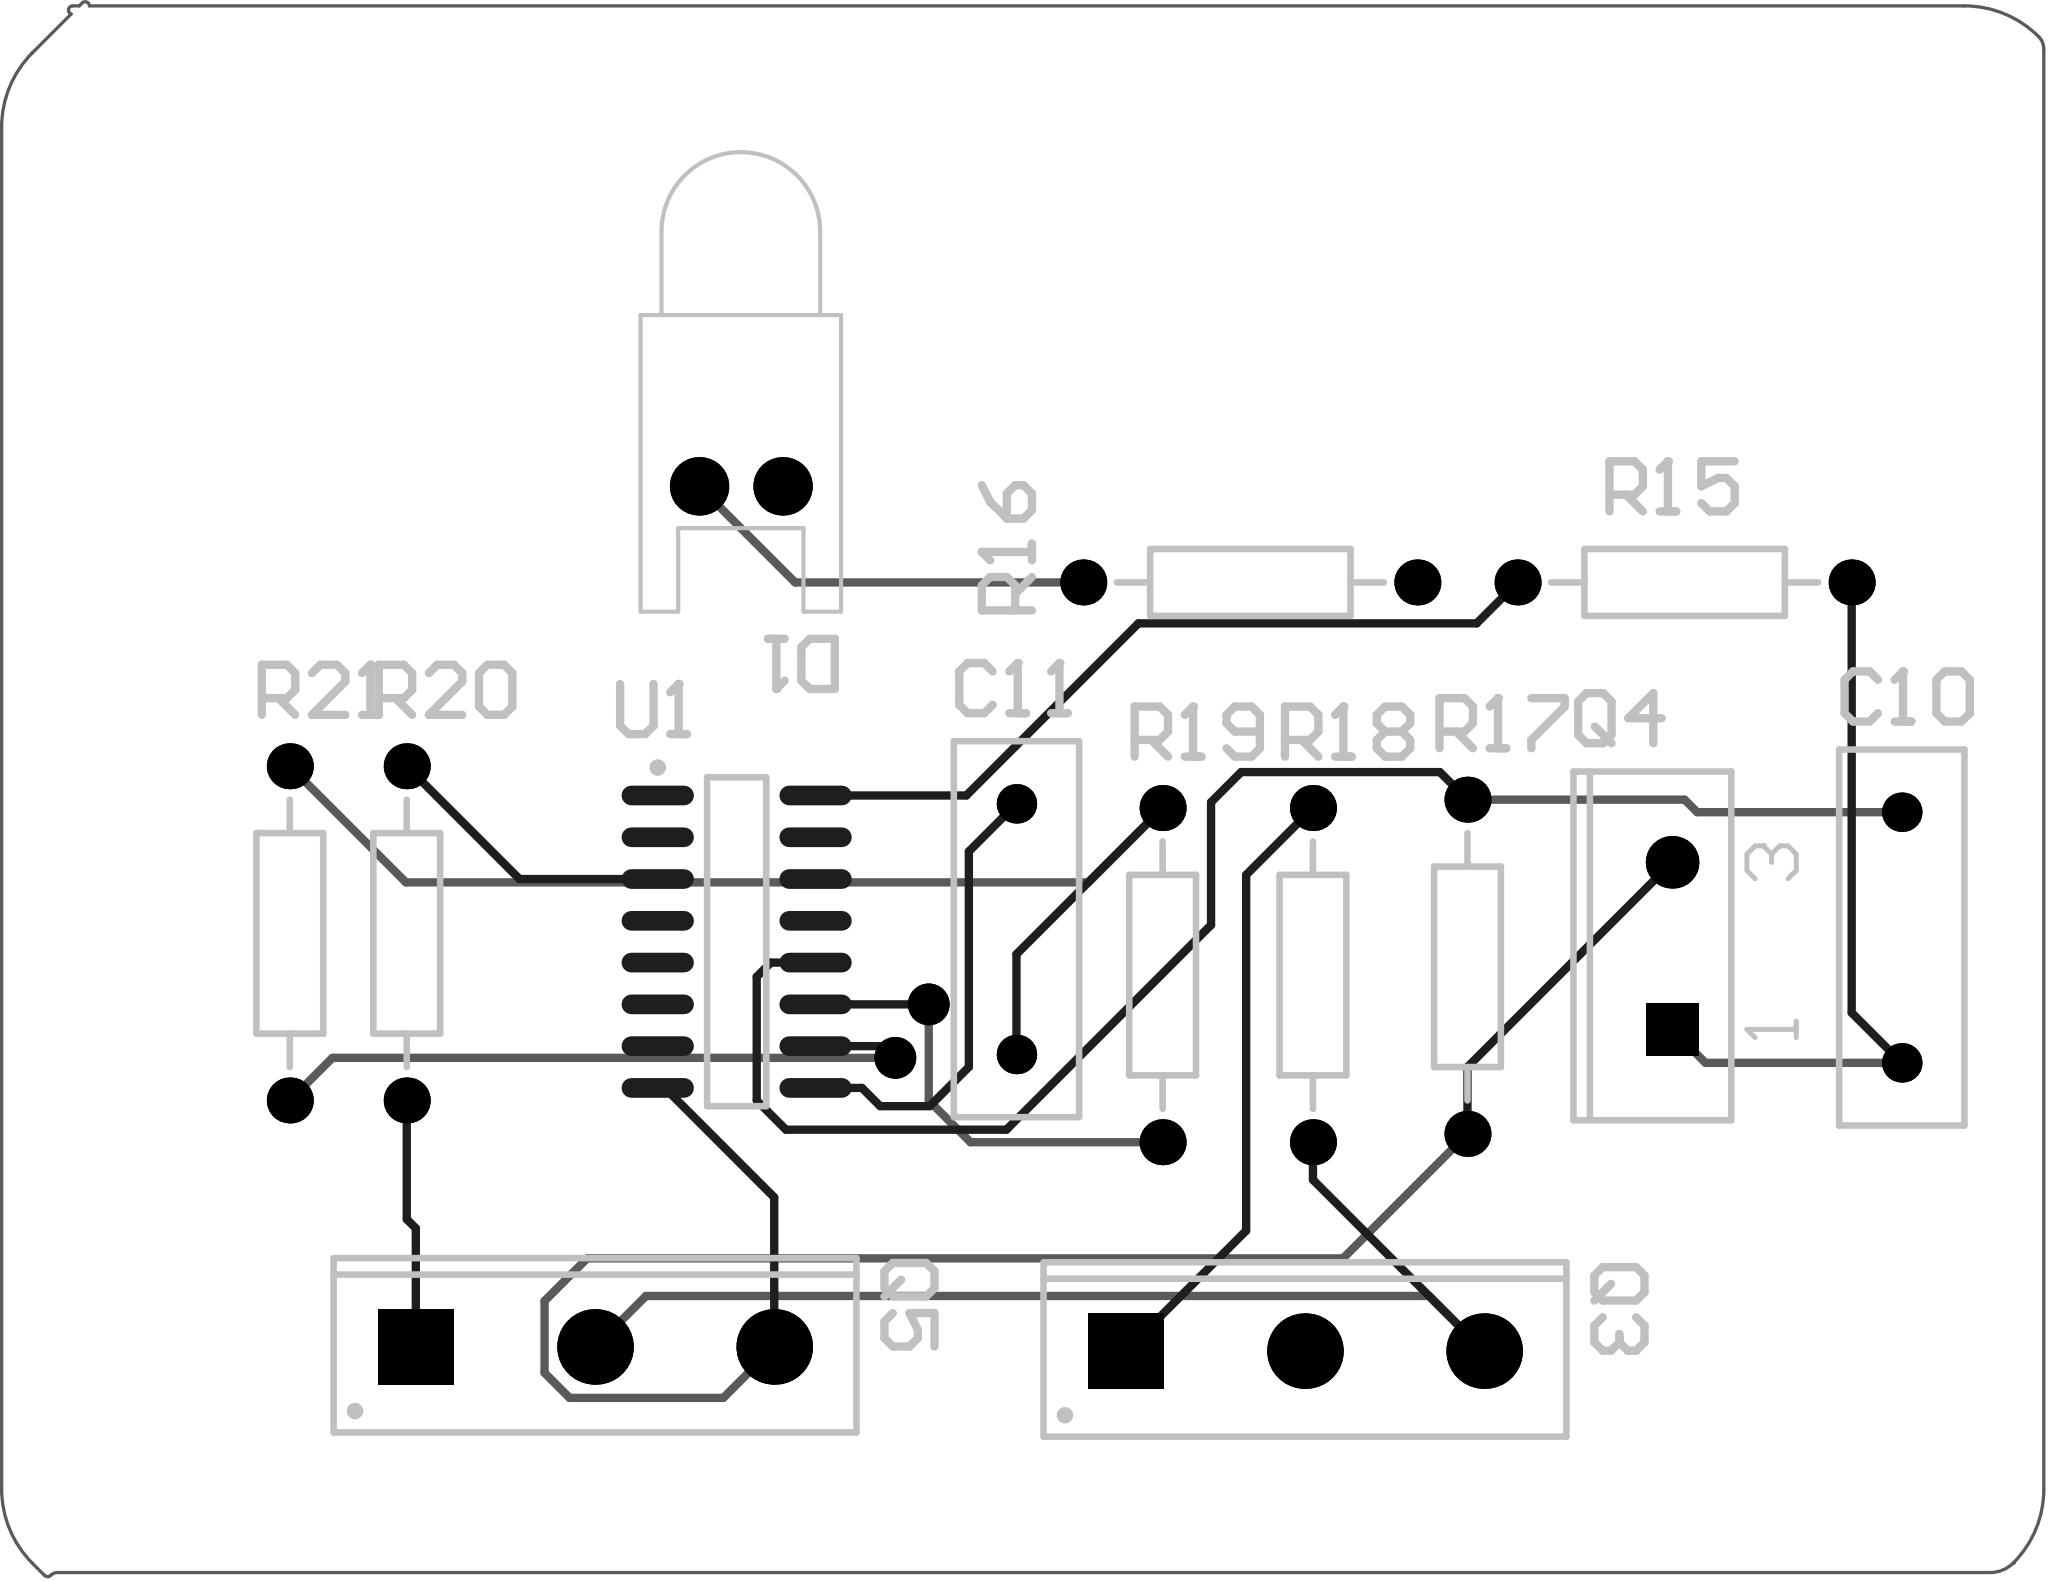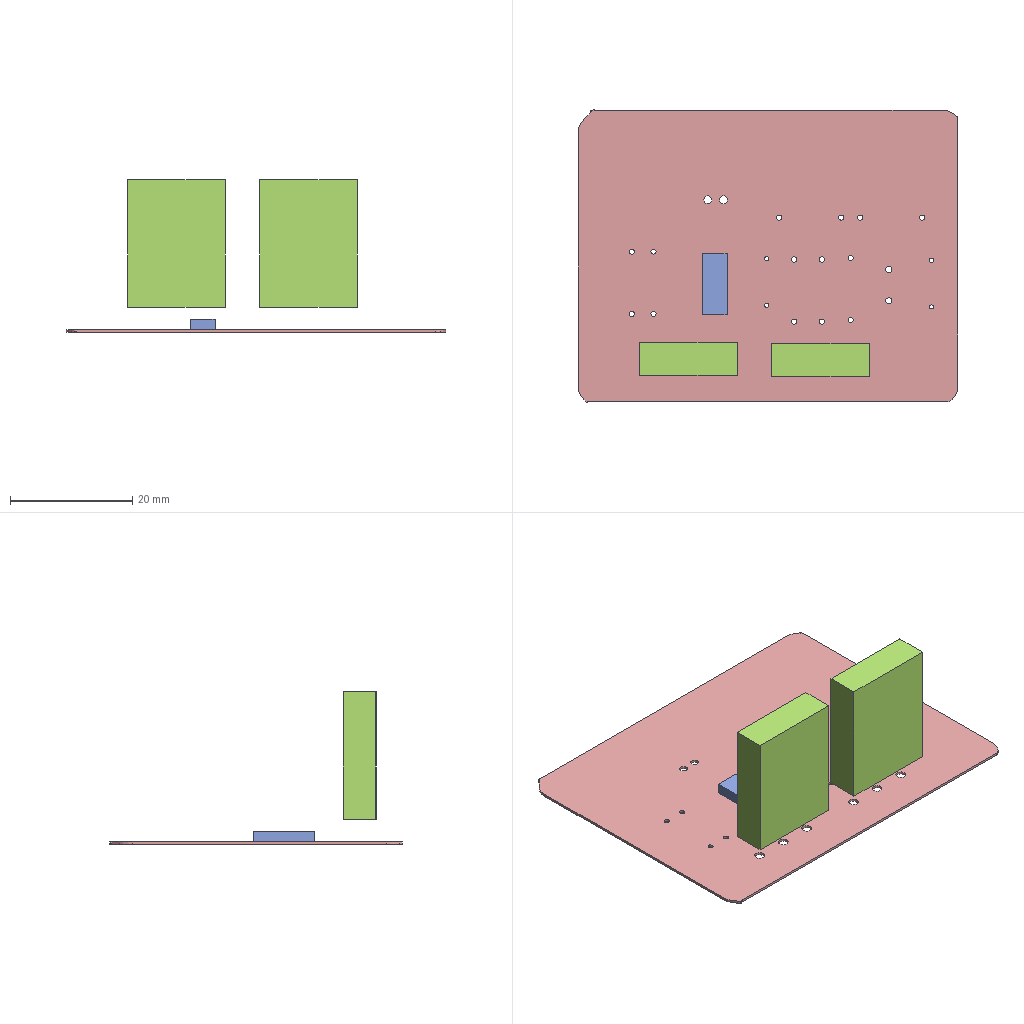Circuit board layout | Altium Designer | box 62.1 x 47.9 x 25 mm
Part placement:
Designator,Comment,Layer,Footprint,Center-X(mm),Center-Y(mm),Rotation
U1,CD4060BCM,TopLayer,M16A_N,95.504,69.85,0
R21,Res2,TopLayer,AXIAL-0.4,81.915,70.104,90
R20,Res2,TopLayer,AXIAL-0.4,85.471,70.104,90
R19,Res2,TopLayer,AXIAL-0.4,108.458,68.834,90
R18,Res2,TopLayer,AXIAL-0.4,113.03,68.834,90
R17,Res2,TopLayer,AXIAL-0.4,117.729,69.088,90
R16,Res2,TopLayer,AXIAL-0.4,111.125,80.772,180
R15,Res2,TopLayer,AXIAL-0.4,124.333,80.772,360
Q5,IRFP044N,TopLayer,TO-247AC,91.197,57.531,360
Q4,Photo NPN,TopLayer,TO-220_A,123.952,69.723,90
Q3,IRFP044N,TopLayer,TO-247AC,112.787,57.404,360
D1,LED0,TopLayer,LED-0,95.631,83.693,180
C11,Cap,TopLayer,RAD-0.3,104.013,70.231,90
C10,Cap,TopLayer,RAD-0.3,130.937,69.977,90